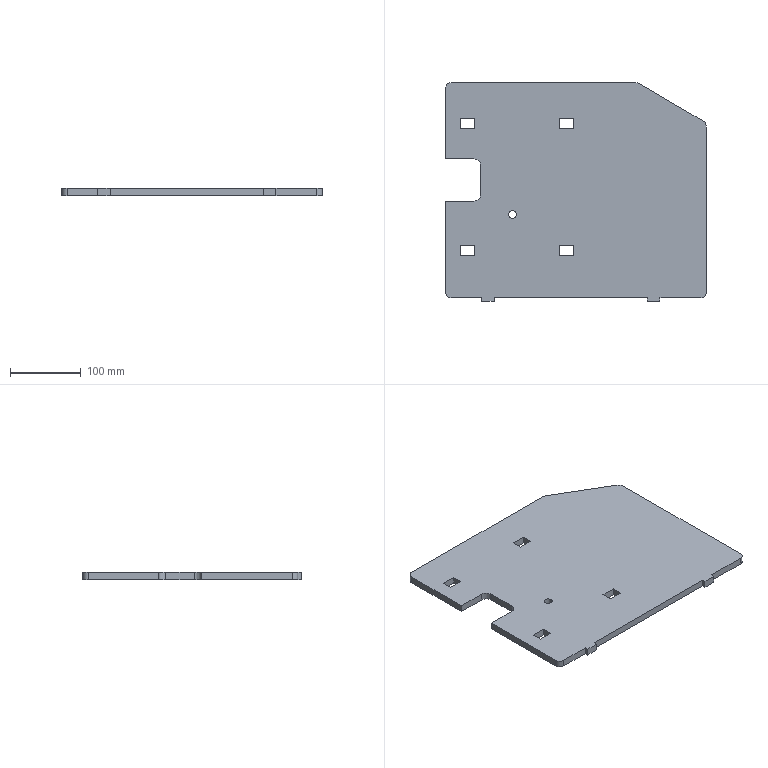Part | SolidWorks | features Extrusion 1 | 1 solid | 44 faces | box 370 x 310 x 10 mm | volume 1059963 mm3 | plane 35 | cylinder 9 | commonest cylinder face diameters 20 x4 16 x3 11 x2
STEP:
#1=CARTESIAN_POINT('',(352.502,683.941,10.));
#2=VERTEX_POINT('',#1);
#3=CARTESIAN_POINT('',(363.502,683.941,10.));
#4=VERTEX_POINT('',#3);
#5=CARTESIAN_POINT('',(358.002,683.941,10.));
#6=DIRECTION('',(0.,0.,1.));
#7=DIRECTION('',(1.,0.,0.));
#8=AXIS2_PLACEMENT_3D('',#5,#6,#7);
#9=CIRCLE('',#8,5.5);
#10=EDGE_CURVE('',#2,#4,#9,.T.);
#11=ORIENTED_EDGE('',*,*,#10,.T.);
#12=CARTESIAN_POINT('',(363.502,683.941,0.));
#13=VERTEX_POINT('',#12);
#14=CARTESIAN_POINT('',(363.502,683.941,10.));
#15=DIRECTION('',(0.,0.,-1.));
#16=VECTOR('',#15,1000.);
#17=LINE('',#14,#16);
#18=EDGE_CURVE('',#4,#13,#17,.T.);
#19=ORIENTED_EDGE('',*,*,#18,.T.);
#20=CARTESIAN_POINT('',(352.502,683.941,0.));
#21=VERTEX_POINT('',#20);
#22=CARTESIAN_POINT('',(358.002,683.941,0.));
#23=DIRECTION('',(0.,0.,1.));
#24=DIRECTION('',(1.,0.,0.));
#25=AXIS2_PLACEMENT_3D('',#22,#23,#24);
#26=CIRCLE('',#25,5.5);
#27=EDGE_CURVE('',#21,#13,#26,.T.);
#28=ORIENTED_EDGE('',*,*,#27,.F.);
#29=CARTESIAN_POINT('',(352.502,683.941,10.));
#30=DIRECTION('',(0.,0.,-1.));
#31=VECTOR('',#30,1000.);
#32=LINE('',#29,#31);
#33=EDGE_CURVE('',#2,#21,#32,.T.);
#34=ORIENTED_EDGE('',*,*,#33,.F.);
#35=EDGE_LOOP('',(#11,#19,#28,#34));
#36=FACE_OUTER_BOUND('',#35,.T.);
#37=CARTESIAN_POINT('',(358.002,683.941,10.));
#38=DIRECTION('',(0.,0.,-1.));
#39=DIRECTION('',(-1.,0.,0.));
#40=AXIS2_PLACEMENT_3D('',#37,#38,#39);
#41=CYLINDRICAL_SURFACE('',#40,5.5);
#42=ADVANCED_FACE('',(#36),#41,.F.);
#43=CARTESIAN_POINT('',(444.202,805.941,10.));
#44=VERTEX_POINT('',#43);
#45=CARTESIAN_POINT('',(444.202,820.141,10.));
#46=VERTEX_POINT('',#45);
#47=CARTESIAN_POINT('',(444.202,820.141,10.));
#48=DIRECTION('',(0.,1.,0.));
#49=VECTOR('',#48,1000.);
#50=LINE('',#47,#49);
#51=EDGE_CURVE('',#44,#46,#50,.T.);
#52=ORIENTED_EDGE('',*,*,#51,.F.);
#53=CARTESIAN_POINT('',(424.002,805.941,10.));
#54=VERTEX_POINT('',#53);
#55=CARTESIAN_POINT('',(444.202,805.941,10.));
#56=DIRECTION('',(1.,0.,0.));
#57=VECTOR('',#56,1000.);
#58=LINE('',#55,#57);
#59=EDGE_CURVE('',#54,#44,#58,.T.);
#60=ORIENTED_EDGE('',*,*,#59,.F.);
#61=CARTESIAN_POINT('',(424.002,820.141,10.));
#62=VERTEX_POINT('',#61);
#63=CARTESIAN_POINT('',(424.002,805.941,10.));
#64=DIRECTION('',(0.,-1.,0.));
#65=VECTOR('',#64,1000.);
#66=LINE('',#63,#65);
#67=EDGE_CURVE('',#62,#54,#66,.T.);
#68=ORIENTED_EDGE('',*,*,#67,.F.);
#69=CARTESIAN_POINT('',(424.002,820.141,10.));
#70=DIRECTION('',(-1.,0.,0.));
#71=VECTOR('',#70,1000.);
#72=LINE('',#69,#71);
#73=EDGE_CURVE('',#46,#62,#72,.T.);
#74=ORIENTED_EDGE('',*,*,#73,.F.);
#75=EDGE_LOOP('',(#52,#60,#68,#74));
#76=FACE_BOUND('',#75,.T.);
#77=CARTESIAN_POINT('',(304.202,805.941,10.));
#78=VERTEX_POINT('',#77);
#79=CARTESIAN_POINT('',(304.202,820.141,10.));
#80=VERTEX_POINT('',#79);
#81=CARTESIAN_POINT('',(304.202,820.141,10.));
#82=DIRECTION('',(0.,1.,0.));
#83=VECTOR('',#82,1000.);
#84=LINE('',#81,#83);
#85=EDGE_CURVE('',#78,#80,#84,.T.);
#86=ORIENTED_EDGE('',*,*,#85,.F.);
#87=CARTESIAN_POINT('',(284.002,805.941,10.));
#88=VERTEX_POINT('',#87);
#89=CARTESIAN_POINT('',(304.202,805.941,10.));
#90=DIRECTION('',(1.,0.,0.));
#91=VECTOR('',#90,1000.);
#92=LINE('',#89,#91);
#93=EDGE_CURVE('',#88,#78,#92,.T.);
#94=ORIENTED_EDGE('',*,*,#93,.F.);
#95=CARTESIAN_POINT('',(284.002,820.141,10.));
#96=VERTEX_POINT('',#95);
#97=CARTESIAN_POINT('',(284.002,805.941,10.));
#98=DIRECTION('',(0.,-1.,0.));
#99=VECTOR('',#98,1000.);
#100=LINE('',#97,#99);
#101=EDGE_CURVE('',#96,#88,#100,.T.);
#102=ORIENTED_EDGE('',*,*,#101,.F.);
#103=CARTESIAN_POINT('',(284.002,820.141,10.));
#104=DIRECTION('',(-1.,0.,0.));
#105=VECTOR('',#104,1000.);
#106=LINE('',#103,#105);
#107=EDGE_CURVE('',#80,#96,#106,.T.);
#108=ORIENTED_EDGE('',*,*,#107,.F.);
#109=EDGE_LOOP('',(#86,#94,#102,#108));
#110=FACE_BOUND('',#109,.T.);
#111=CARTESIAN_POINT('',(444.202,626.141,10.));
#112=VERTEX_POINT('',#111);
#113=CARTESIAN_POINT('',(444.202,640.341,10.));
#114=VERTEX_POINT('',#113);
#115=CARTESIAN_POINT('',(444.202,640.341,10.));
#116=DIRECTION('',(0.,1.,0.));
#117=VECTOR('',#116,1000.);
#118=LINE('',#115,#117);
#119=EDGE_CURVE('',#112,#114,#118,.T.);
#120=ORIENTED_EDGE('',*,*,#119,.F.);
#121=CARTESIAN_POINT('',(424.002,626.141,10.));
#122=VERTEX_POINT('',#121);
#123=CARTESIAN_POINT('',(444.202,626.141,10.));
#124=DIRECTION('',(1.,0.,0.));
#125=VECTOR('',#124,1000.);
#126=LINE('',#123,#125);
#127=EDGE_CURVE('',#122,#112,#126,.T.);
#128=ORIENTED_EDGE('',*,*,#127,.F.);
#129=CARTESIAN_POINT('',(424.002,640.341,10.));
#130=VERTEX_POINT('',#129);
#131=CARTESIAN_POINT('',(424.002,626.141,10.));
#132=DIRECTION('',(0.,-1.,0.));
#133=VECTOR('',#132,1000.);
#134=LINE('',#131,#133);
#135=EDGE_CURVE('',#130,#122,#134,.T.);
#136=ORIENTED_EDGE('',*,*,#135,.F.);
#137=CARTESIAN_POINT('',(424.002,640.341,10.));
#138=DIRECTION('',(-1.,0.,0.));
#139=VECTOR('',#138,1000.);
#140=LINE('',#137,#139);
#141=EDGE_CURVE('',#114,#130,#140,.T.);
#142=ORIENTED_EDGE('',*,*,#141,.F.);
#143=EDGE_LOOP('',(#120,#128,#136,#142));
#144=FACE_BOUND('',#143,.T.);
#145=CARTESIAN_POINT('',(304.202,626.141,10.));
#146=VERTEX_POINT('',#145);
#147=CARTESIAN_POINT('',(304.202,640.341,10.));
#148=VERTEX_POINT('',#147);
#149=CARTESIAN_POINT('',(304.202,640.341,10.));
#150=DIRECTION('',(0.,1.,0.));
#151=VECTOR('',#150,1000.);
#152=LINE('',#149,#151);
#153=EDGE_CURVE('',#146,#148,#152,.T.);
#154=ORIENTED_EDGE('',*,*,#153,.F.);
#155=CARTESIAN_POINT('',(284.002,626.141,10.));
#156=VERTEX_POINT('',#155);
#157=CARTESIAN_POINT('',(304.202,626.141,10.));
#158=DIRECTION('',(1.,0.,0.));
#159=VECTOR('',#158,1000.);
#160=LINE('',#157,#159);
#161=EDGE_CURVE('',#156,#146,#160,.T.);
#162=ORIENTED_EDGE('',*,*,#161,.F.);
#163=CARTESIAN_POINT('',(284.002,640.341,10.));
#164=VERTEX_POINT('',#163);
#165=CARTESIAN_POINT('',(284.002,626.141,10.));
#166=DIRECTION('',(0.,-1.,0.));
#167=VECTOR('',#166,1000.);
#168=LINE('',#165,#167);
#169=EDGE_CURVE('',#164,#156,#168,.T.);
#170=ORIENTED_EDGE('',*,*,#169,.F.);
#171=CARTESIAN_POINT('',(284.002,640.341,10.));
#172=DIRECTION('',(-1.,0.,0.));
#173=VECTOR('',#172,1000.);
#174=LINE('',#171,#173);
#175=EDGE_CURVE('',#148,#164,#174,.T.);
#176=ORIENTED_EDGE('',*,*,#175,.F.);
#177=EDGE_LOOP('',(#154,#162,#170,#176));
#178=FACE_BOUND('',#177,.T.);
#179=CARTESIAN_POINT('',(633.002,807.92,10.));
#180=VERTEX_POINT('',#179);
#181=CARTESIAN_POINT('',(628.108,816.518,10.));
#182=VERTEX_POINT('',#181);
#183=CARTESIAN_POINT('',(623.002,807.92,10.));
#184=DIRECTION('',(0.,0.,1.));
#185=DIRECTION('',(1.,0.,0.));
#186=AXIS2_PLACEMENT_3D('',#183,#184,#185);
#187=CIRCLE('',#186,10.);
#188=EDGE_CURVE('',#180,#182,#187,.T.);
#189=ORIENTED_EDGE('',*,*,#188,.T.);
#190=CARTESIAN_POINT('',(538.108,869.539,10.));
#191=VERTEX_POINT('',#190);
#192=CARTESIAN_POINT('',(538.108,869.539,10.));
#193=DIRECTION('',(-0.8616,0.5076,0.));
#194=VECTOR('',#193,1000.);
#195=LINE('',#192,#194);
#196=EDGE_CURVE('',#182,#191,#195,.T.);
#197=ORIENTED_EDGE('',*,*,#196,.T.);
#198=CARTESIAN_POINT('',(533.002,870.941,10.));
#199=VERTEX_POINT('',#198);
#200=CARTESIAN_POINT('',(533.002,860.941,10.));
#201=DIRECTION('',(0.,0.,1.));
#202=DIRECTION('',(1.,0.,0.));
#203=AXIS2_PLACEMENT_3D('',#200,#201,#202);
#204=CIRCLE('',#203,10.);
#205=EDGE_CURVE('',#191,#199,#204,.T.);
#206=ORIENTED_EDGE('',*,*,#205,.T.);
#207=CARTESIAN_POINT('',(271.002,870.941,10.));
#208=VERTEX_POINT('',#207);
#209=CARTESIAN_POINT('',(533.002,870.941,10.));
#210=DIRECTION('',(-1.,0.,0.));
#211=VECTOR('',#210,1000.);
#212=LINE('',#209,#211);
#213=EDGE_CURVE('',#199,#208,#212,.T.);
#214=ORIENTED_EDGE('',*,*,#213,.T.);
#215=CARTESIAN_POINT('',(263.002,862.941,10.));
#216=VERTEX_POINT('',#215);
#217=CARTESIAN_POINT('',(271.002,862.941,10.));
#218=DIRECTION('',(0.,0.,1.));
#219=DIRECTION('',(1.,0.,0.));
#220=AXIS2_PLACEMENT_3D('',#217,#218,#219);
#221=CIRCLE('',#220,8.);
#222=EDGE_CURVE('',#208,#216,#221,.T.);
#223=ORIENTED_EDGE('',*,*,#222,.T.);
#224=CARTESIAN_POINT('',(263.002,762.941,10.));
#225=VERTEX_POINT('',#224);
#226=CARTESIAN_POINT('',(263.002,862.941,10.));
#227=DIRECTION('',(0.,-1.,0.));
#228=VECTOR('',#227,1000.);
#229=LINE('',#226,#228);
#230=EDGE_CURVE('',#216,#225,#229,.T.);
#231=ORIENTED_EDGE('',*,*,#230,.T.);
#232=CARTESIAN_POINT('',(303.002,762.941,10.));
#233=VERTEX_POINT('',#232);
#234=CARTESIAN_POINT('',(263.002,762.941,10.));
#235=DIRECTION('',(1.,0.,0.));
#236=VECTOR('',#235,1000.);
#237=LINE('',#234,#236);
#238=EDGE_CURVE('',#225,#233,#237,.T.);
#239=ORIENTED_EDGE('',*,*,#238,.T.);
#240=CARTESIAN_POINT('',(313.002,752.941,10.));
#241=VERTEX_POINT('',#240);
#242=CARTESIAN_POINT('',(303.002,752.941,10.));
#243=DIRECTION('',(0.,0.,-1.));
#244=DIRECTION('',(1.,0.,0.));
#245=AXIS2_PLACEMENT_3D('',#242,#243,#244);
#246=CIRCLE('',#245,10.);
#247=EDGE_CURVE('',#233,#241,#246,.T.);
#248=ORIENTED_EDGE('',*,*,#247,.T.);
#249=CARTESIAN_POINT('',(313.002,712.941,10.));
#250=VERTEX_POINT('',#249);
#251=CARTESIAN_POINT('',(313.002,752.941,10.));
#252=DIRECTION('',(0.,-1.,0.));
#253=VECTOR('',#252,1000.);
#254=LINE('',#251,#253);
#255=EDGE_CURVE('',#241,#250,#254,.T.);
#256=ORIENTED_EDGE('',*,*,#255,.T.);
#257=CARTESIAN_POINT('',(303.002,702.941,10.));
#258=VERTEX_POINT('',#257);
#259=CARTESIAN_POINT('',(303.002,712.941,10.));
#260=DIRECTION('',(0.,0.,-1.));
#261=DIRECTION('',(1.,0.,0.));
#262=AXIS2_PLACEMENT_3D('',#259,#260,#261);
#263=CIRCLE('',#262,10.);
#264=EDGE_CURVE('',#250,#258,#263,.T.);
#265=ORIENTED_EDGE('',*,*,#264,.T.);
#266=CARTESIAN_POINT('',(263.002,702.941,10.));
#267=VERTEX_POINT('',#266);
#268=CARTESIAN_POINT('',(303.002,702.941,10.));
#269=DIRECTION('',(-1.,0.,0.));
#270=VECTOR('',#269,1000.);
#271=LINE('',#268,#270);
#272=EDGE_CURVE('',#258,#267,#271,.T.);
#273=ORIENTED_EDGE('',*,*,#272,.T.);
#274=CARTESIAN_POINT('',(263.002,573.941,10.));
#275=VERTEX_POINT('',#274);
#276=CARTESIAN_POINT('',(263.002,702.941,10.));
#277=DIRECTION('',(0.,-1.,0.));
#278=VECTOR('',#277,1000.);
#279=LINE('',#276,#278);
#280=EDGE_CURVE('',#267,#275,#279,.T.);
#281=ORIENTED_EDGE('',*,*,#280,.T.);
#282=CARTESIAN_POINT('',(271.002,565.941,10.));
#283=VERTEX_POINT('',#282);
#284=CARTESIAN_POINT('',(271.002,573.941,10.));
#285=DIRECTION('',(0.,0.,1.));
#286=DIRECTION('',(1.,0.,0.));
#287=AXIS2_PLACEMENT_3D('',#284,#285,#286);
#288=CIRCLE('',#287,8.);
#289=EDGE_CURVE('',#275,#283,#288,.T.);
#290=ORIENTED_EDGE('',*,*,#289,.T.);
#291=CARTESIAN_POINT('',(314.061,565.941,10.));
#292=VERTEX_POINT('',#291);
#293=CARTESIAN_POINT('',(271.002,565.941,10.));
#294=DIRECTION('',(1.,0.,0.));
#295=VECTOR('',#294,1000.);
#296=LINE('',#293,#295);
#297=EDGE_CURVE('',#283,#292,#296,.T.);
#298=ORIENTED_EDGE('',*,*,#297,.T.);
#299=CARTESIAN_POINT('',(314.061,560.941,10.));
#300=VERTEX_POINT('',#299);
#301=CARTESIAN_POINT('',(314.061,565.941,10.));
#302=DIRECTION('',(0.,-1.,0.));
#303=VECTOR('',#302,1000.);
#304=LINE('',#301,#303);
#305=EDGE_CURVE('',#292,#300,#304,.T.);
#306=ORIENTED_EDGE('',*,*,#305,.T.);
#307=CARTESIAN_POINT('',(332.061,560.941,10.));
#308=VERTEX_POINT('',#307);
#309=CARTESIAN_POINT('',(314.061,560.941,10.));
#310=DIRECTION('',(1.,0.,0.));
#311=VECTOR('',#310,1000.);
#312=LINE('',#309,#311);
#313=EDGE_CURVE('',#300,#308,#312,.T.);
#314=ORIENTED_EDGE('',*,*,#313,.T.);
#315=CARTESIAN_POINT('',(332.061,565.941,10.));
#316=VERTEX_POINT('',#315);
#317=CARTESIAN_POINT('',(332.061,560.941,10.));
#318=DIRECTION('',(0.,1.,0.));
#319=VECTOR('',#318,1000.);
#320=LINE('',#317,#319);
#321=EDGE_CURVE('',#308,#316,#320,.T.);
#322=ORIENTED_EDGE('',*,*,#321,.T.);
#323=CARTESIAN_POINT('',(549.061,565.941,10.));
#324=VERTEX_POINT('',#323);
#325=CARTESIAN_POINT('',(332.061,565.941,10.));
#326=DIRECTION('',(1.,0.,0.));
#327=VECTOR('',#326,1000.);
#328=LINE('',#325,#327);
#329=EDGE_CURVE('',#316,#324,#328,.T.);
#330=ORIENTED_EDGE('',*,*,#329,.T.);
#331=CARTESIAN_POINT('',(549.061,560.941,10.));
#332=VERTEX_POINT('',#331);
#333=CARTESIAN_POINT('',(549.061,565.941,10.));
#334=DIRECTION('',(0.,-1.,0.));
#335=VECTOR('',#334,1000.);
#336=LINE('',#333,#335);
#337=EDGE_CURVE('',#324,#332,#336,.T.);
#338=ORIENTED_EDGE('',*,*,#337,.T.);
#339=CARTESIAN_POINT('',(567.061,560.941,10.));
#340=VERTEX_POINT('',#339);
#341=CARTESIAN_POINT('',(549.061,560.941,10.));
#342=DIRECTION('',(1.,0.,0.));
#343=VECTOR('',#342,1000.);
#344=LINE('',#341,#343);
#345=EDGE_CURVE('',#332,#340,#344,.T.);
#346=ORIENTED_EDGE('',*,*,#345,.T.);
#347=CARTESIAN_POINT('',(567.061,565.941,10.));
#348=VERTEX_POINT('',#347);
#349=CARTESIAN_POINT('',(567.061,560.941,10.));
#350=DIRECTION('',(0.,1.,0.));
#351=VECTOR('',#350,1000.);
#352=LINE('',#349,#351);
#353=EDGE_CURVE('',#340,#348,#352,.T.);
#354=ORIENTED_EDGE('',*,*,#353,.T.);
#355=CARTESIAN_POINT('',(625.002,565.941,10.));
#356=VERTEX_POINT('',#355);
#357=CARTESIAN_POINT('',(567.061,565.941,10.));
#358=DIRECTION('',(1.,0.,0.));
#359=VECTOR('',#358,1000.);
#360=LINE('',#357,#359);
#361=EDGE_CURVE('',#348,#356,#360,.T.);
#362=ORIENTED_EDGE('',*,*,#361,.T.);
#363=CARTESIAN_POINT('',(633.002,573.941,10.));
#364=VERTEX_POINT('',#363);
#365=CARTESIAN_POINT('',(625.002,573.941,10.));
#366=DIRECTION('',(0.,0.,1.));
#367=DIRECTION('',(1.,0.,0.));
#368=AXIS2_PLACEMENT_3D('',#365,#366,#367);
#369=CIRCLE('',#368,8.);
#370=EDGE_CURVE('',#356,#364,#369,.T.);
#371=ORIENTED_EDGE('',*,*,#370,.T.);
#372=CARTESIAN_POINT('',(633.002,807.92,10.));
#373=DIRECTION('',(0.,1.,0.));
#374=VECTOR('',#373,1000.);
#375=LINE('',#372,#374);
#376=EDGE_CURVE('',#364,#180,#375,.T.);
#377=ORIENTED_EDGE('',*,*,#376,.T.);
#378=EDGE_LOOP('',(#189,#197,#206,#214,#223,#231,#239,#248,#256,#265,#273,#281,#290,#298,#306,#314,#322,#330,#338,#346,#354,#362,#371,#377));
#379=FACE_OUTER_BOUND('',#378,.T.);
#380=ORIENTED_EDGE('',*,*,#10,.F.);
#381=CARTESIAN_POINT('',(358.002,683.941,10.));
#382=DIRECTION('',(0.,0.,1.));
#383=DIRECTION('',(1.,0.,0.));
#384=AXIS2_PLACEMENT_3D('',#381,#382,#383);
#385=CIRCLE('',#384,5.5);
#386=EDGE_CURVE('',#4,#2,#385,.T.);
#387=ORIENTED_EDGE('',*,*,#386,.F.);
#388=EDGE_LOOP('',(#380,#387));
#389=FACE_BOUND('',#388,.T.);
#390=CARTESIAN_POINT('',(623.002,807.92,10.));
#391=DIRECTION('',(0.,0.,1.));
#392=DIRECTION('',(1.,0.,0.));
#393=AXIS2_PLACEMENT_3D('',#390,#391,#392);
#394=PLANE('',#393);
#395=ADVANCED_FACE('',(#76,#110,#144,#178,#379,#389),#394,.T.);
#396=CARTESIAN_POINT('',(284.002,805.941,0.));
#397=VERTEX_POINT('',#396);
#398=CARTESIAN_POINT('',(304.202,805.941,0.));
#399=VERTEX_POINT('',#398);
#400=CARTESIAN_POINT('',(304.202,805.941,0.));
#401=DIRECTION('',(1.,0.,0.));
#402=VECTOR('',#401,1000.);
#403=LINE('',#400,#402);
#404=EDGE_CURVE('',#397,#399,#403,.T.);
#405=ORIENTED_EDGE('',*,*,#404,.T.);
#406=CARTESIAN_POINT('',(304.202,820.141,0.));
#407=VERTEX_POINT('',#406);
#408=CARTESIAN_POINT('',(304.202,820.141,0.));
#409=DIRECTION('',(0.,1.,0.));
#410=VECTOR('',#409,1000.);
#411=LINE('',#408,#410);
#412=EDGE_CURVE('',#399,#407,#411,.T.);
#413=ORIENTED_EDGE('',*,*,#412,.T.);
#414=CARTESIAN_POINT('',(284.002,820.141,0.));
#415=VERTEX_POINT('',#414);
#416=CARTESIAN_POINT('',(284.002,820.141,0.));
#417=DIRECTION('',(-1.,0.,0.));
#418=VECTOR('',#417,1000.);
#419=LINE('',#416,#418);
#420=EDGE_CURVE('',#407,#415,#419,.T.);
#421=ORIENTED_EDGE('',*,*,#420,.T.);
#422=CARTESIAN_POINT('',(284.002,805.941,0.));
#423=DIRECTION('',(0.,-1.,0.));
#424=VECTOR('',#423,1000.);
#425=LINE('',#422,#424);
#426=EDGE_CURVE('',#415,#397,#425,.T.);
#427=ORIENTED_EDGE('',*,*,#426,.T.);
#428=EDGE_LOOP('',(#405,#413,#421,#427));
#429=FACE_BOUND('',#428,.T.);
#430=CARTESIAN_POINT('',(284.002,626.141,0.));
#431=VERTEX_POINT('',#430);
#432=CARTESIAN_POINT('',(304.202,626.141,0.));
#433=VERTEX_POINT('',#432);
#434=CARTESIAN_POINT('',(304.202,626.141,0.));
#435=DIRECTION('',(1.,0.,0.));
#436=VECTOR('',#435,1000.);
#437=LINE('',#434,#436);
#438=EDGE_CURVE('',#431,#433,#437,.T.);
#439=ORIENTED_EDGE('',*,*,#438,.T.);
#440=CARTESIAN_POINT('',(304.202,640.341,0.));
#441=VERTEX_POINT('',#440);
#442=CARTESIAN_POINT('',(304.202,640.341,0.));
#443=DIRECTION('',(0.,1.,0.));
#444=VECTOR('',#443,1000.);
#445=LINE('',#442,#444);
#446=EDGE_CURVE('',#433,#441,#445,.T.);
#447=ORIENTED_EDGE('',*,*,#446,.T.);
#448=CARTESIAN_POINT('',(284.002,640.341,0.));
#449=VERTEX_POINT('',#448);
#450=CARTESIAN_POINT('',(284.002,640.341,0.));
#451=DIRECTION('',(-1.,0.,0.));
#452=VECTOR('',#451,1000.);
#453=LINE('',#450,#452);
#454=EDGE_CURVE('',#441,#449,#453,.T.);
#455=ORIENTED_EDGE('',*,*,#454,.T.);
#456=CARTESIAN_POINT('',(284.002,626.141,0.));
#457=DIRECTION('',(0.,-1.,0.));
#458=VECTOR('',#457,1000.);
#459=LINE('',#456,#458);
#460=EDGE_CURVE('',#449,#431,#459,.T.);
#461=ORIENTED_EDGE('',*,*,#460,.T.);
#462=EDGE_LOOP('',(#439,#447,#455,#461));
#463=FACE_BOUND('',#462,.T.);
#464=CARTESIAN_POINT('',(633.002,807.92,0.));
#465=VERTEX_POINT('',#464);
#466=CARTESIAN_POINT('',(628.108,816.518,0.));
#467=VERTEX_POINT('',#466);
#468=CARTESIAN_POINT('',(623.002,807.92,0.));
#469=DIRECTION('',(0.,0.,1.));
#470=DIRECTION('',(1.,0.,0.));
#471=AXIS2_PLACEMENT_3D('',#468,#469,#470);
#472=CIRCLE('',#471,10.);
#473=EDGE_CURVE('',#465,#467,#472,.T.);
#474=ORIENTED_EDGE('',*,*,#473,.F.);
#475=CARTESIAN_POINT('',(633.002,573.941,0.));
#476=VERTEX_POINT('',#475);
#477=CARTESIAN_POINT('',(633.002,807.92,0.));
#478=DIRECTION('',(0.,1.,0.));
#479=VECTOR('',#478,1000.);
#480=LINE('',#477,#479);
#481=EDGE_CURVE('',#476,#465,#480,.T.);
#482=ORIENTED_EDGE('',*,*,#481,.F.);
#483=CARTESIAN_POINT('',(625.002,565.941,0.));
#484=VERTEX_POINT('',#483);
#485=CARTESIAN_POINT('',(625.002,573.941,0.));
#486=DIRECTION('',(0.,0.,1.));
#487=DIRECTION('',(1.,0.,0.));
#488=AXIS2_PLACEMENT_3D('',#485,#486,#487);
#489=CIRCLE('',#488,8.);
#490=EDGE_CURVE('',#484,#476,#489,.T.);
#491=ORIENTED_EDGE('',*,*,#490,.F.);
#492=CARTESIAN_POINT('',(567.061,565.941,0.));
#493=VERTEX_POINT('',#492);
#494=CARTESIAN_POINT('',(567.061,565.941,0.));
#495=DIRECTION('',(1.,0.,0.));
#496=VECTOR('',#495,1000.);
#497=LINE('',#494,#496);
#498=EDGE_CURVE('',#493,#484,#497,.T.);
#499=ORIENTED_EDGE('',*,*,#498,.F.);
#500=CARTESIAN_POINT('',(567.061,560.941,0.));
#501=VERTEX_POINT('',#500);
#502=CARTESIAN_POINT('',(567.061,560.941,0.));
#503=DIRECTION('',(0.,1.,0.));
#504=VECTOR('',#503,1000.);
#505=LINE('',#502,#504);
#506=EDGE_CURVE('',#501,#493,#505,.T.);
#507=ORIENTED_EDGE('',*,*,#506,.F.);
#508=CARTESIAN_POINT('',(549.061,560.941,0.));
#509=VERTEX_POINT('',#508);
#510=CARTESIAN_POINT('',(549.061,560.941,0.));
#511=DIRECTION('',(1.,0.,0.));
#512=VECTOR('',#511,1000.);
#513=LINE('',#510,#512);
#514=EDGE_CURVE('',#509,#501,#513,.T.);
#515=ORIENTED_EDGE('',*,*,#514,.F.);
#516=CARTESIAN_POINT('',(549.061,565.941,0.));
#517=VERTEX_POINT('',#516);
#518=CARTESIAN_POINT('',(549.061,565.941,0.));
#519=DIRECTION('',(0.,-1.,0.));
#520=VECTOR('',#519,1000.);
#521=LINE('',#518,#520);
#522=EDGE_CURVE('',#517,#509,#521,.T.);
#523=ORIENTED_EDGE('',*,*,#522,.F.);
#524=CARTESIAN_POINT('',(332.061,565.941,0.));
#525=VERTEX_POINT('',#524);
#526=CARTESIAN_POINT('',(332.061,565.941,0.));
#527=DIRECTION('',(1.,0.,0.));
#528=VECTOR('',#527,1000.);
#529=LINE('',#526,#528);
#530=EDGE_CURVE('',#525,#517,#529,.T.);
#531=ORIENTED_EDGE('',*,*,#530,.F.);
#532=CARTESIAN_POINT('',(332.061,560.941,0.));
#533=VERTEX_POINT('',#532);
#534=CARTESIAN_POINT('',(332.061,560.941,0.));
#535=DIRECTION('',(0.,1.,0.));
#536=VECTOR('',#535,1000.);
#537=LINE('',#534,#536);
#538=EDGE_CURVE('',#533,#525,#537,.T.);
#539=ORIENTED_EDGE('',*,*,#538,.F.);
#540=CARTESIAN_POINT('',(314.061,560.941,0.));
#541=VERTEX_POINT('',#540);
#542=CARTESIAN_POINT('',(314.061,560.941,0.));
#543=DIRECTION('',(1.,0.,0.));
#544=VECTOR('',#543,1000.);
#545=LINE('',#542,#544);
#546=EDGE_CURVE('',#541,#533,#545,.T.);
#547=ORIENTED_EDGE('',*,*,#546,.F.);
#548=CARTESIAN_POINT('',(314.061,565.941,0.));
#549=VERTEX_POINT('',#548);
#550=CARTESIAN_POINT('',(314.061,565.941,0.));
#551=DIRECTION('',(0.,-1.,0.));
#552=VECTOR('',#551,1000.);
#553=LINE('',#550,#552);
#554=EDGE_CURVE('',#549,#541,#553,.T.);
#555=ORIENTED_EDGE('',*,*,#554,.F.);
#556=CARTESIAN_POINT('',(271.002,565.941,0.));
#557=VERTEX_POINT('',#556);
#558=CARTESIAN_POINT('',(271.002,565.941,0.));
#559=DIRECTION('',(1.,0.,0.));
#560=VECTOR('',#559,1000.);
#561=LINE('',#558,#560);
#562=EDGE_CURVE('',#557,#549,#561,.T.);
#563=ORIENTED_EDGE('',*,*,#562,.F.);
#564=CARTESIAN_POINT('',(263.002,573.941,0.));
#565=VERTEX_POINT('',#564);
#566=CARTESIAN_POINT('',(271.002,573.941,0.));
#567=DIRECTION('',(0.,0.,1.));
#568=DIRECTION('',(1.,0.,0.));
#569=AXIS2_PLACEMENT_3D('',#566,#567,#568);
#570=CIRCLE('',#569,8.);
#571=EDGE_CURVE('',#565,#557,#570,.T.);
#572=ORIENTED_EDGE('',*,*,#571,.F.);
#573=CARTESIAN_POINT('',(263.002,702.941,0.));
#574=VERTEX_POINT('',#573);
#575=CARTESIAN_POINT('',(263.002,702.941,0.));
#576=DIRECTION('',(0.,-1.,0.));
#577=VECTOR('',#576,1000.);
#578=LINE('',#575,#577);
#579=EDGE_CURVE('',#574,#565,#578,.T.);
#580=ORIENTED_EDGE('',*,*,#579,.F.);
#581=CARTESIAN_POINT('',(303.002,702.941,0.));
#582=VERTEX_POINT('',#581);
#583=CARTESIAN_POINT('',(303.002,702.941,0.));
#584=DIRECTION('',(-1.,0.,0.));
#585=VECTOR('',#584,1000.);
#586=LINE('',#583,#585);
#587=EDGE_CURVE('',#582,#574,#586,.T.);
#588=ORIENTED_EDGE('',*,*,#587,.F.);
#589=CARTESIAN_POINT('',(313.002,712.941,0.));
#590=VERTEX_POINT('',#589);
#591=CARTESIAN_POINT('',(303.002,712.941,0.));
#592=DIRECTION('',(0.,0.,-1.));
#593=DIRECTION('',(1.,0.,0.));
#594=AXIS2_PLACEMENT_3D('',#591,#592,#593);
#595=CIRCLE('',#594,10.);
#596=EDGE_CURVE('',#590,#582,#595,.T.);
#597=ORIENTED_EDGE('',*,*,#596,.F.);
#598=CARTESIAN_POINT('',(313.002,752.941,0.));
#599=VERTEX_POINT('',#598);
#600=CARTESIAN_POINT('',(313.002,752.941,0.));
#601=DIRECTION('',(0.,-1.,0.));
#602=VECTOR('',#601,1000.);
#603=LINE('',#600,#602);
#604=EDGE_CURVE('',#599,#590,#603,.T.);
#605=ORIENTED_EDGE('',*,*,#604,.F.);
#606=CARTESIAN_POINT('',(303.002,762.941,0.));
#607=VERTEX_POINT('',#606);
#608=CARTESIAN_POINT('',(303.002,752.941,0.));
#609=DIRECTION('',(0.,0.,-1.));
#610=DIRECTION('',(1.,0.,0.));
#611=AXIS2_PLACEMENT_3D('',#608,#609,#610);
#612=CIRCLE('',#611,10.);
#613=EDGE_CURVE('',#607,#599,#612,.T.);
#614=ORIENTED_EDGE('',*,*,#613,.F.);
#615=CARTESIAN_POINT('',(263.002,762.941,0.));
#616=VERTEX_POINT('',#615);
#617=CARTESIAN_POINT('',(263.002,762.941,0.));
#618=DIRECTION('',(1.,0.,0.));
#619=VECTOR('',#618,1000.);
#620=LINE('',#617,#619);
#621=EDGE_CURVE('',#616,#607,#620,.T.);
#622=ORIENTED_EDGE('',*,*,#621,.F.);
#623=CARTESIAN_POINT('',(263.002,862.941,0.));
#624=VERTEX_POINT('',#623);
#625=CARTESIAN_POINT('',(263.002,862.941,0.));
#626=DIRECTION('',(0.,-1.,0.));
#627=VECTOR('',#626,1000.);
#628=LINE('',#625,#627);
#629=EDGE_CURVE('',#624,#616,#628,.T.);
#630=ORIENTED_EDGE('',*,*,#629,.F.);
#631=CARTESIAN_POINT('',(271.002,870.941,0.));
#632=VERTEX_POINT('',#631);
#633=CARTESIAN_POINT('',(271.002,862.941,0.));
#634=DIRECTION('',(0.,0.,1.));
#635=DIRECTION('',(1.,0.,0.));
#636=AXIS2_PLACEMENT_3D('',#633,#634,#635);
#637=CIRCLE('',#636,8.);
#638=EDGE_CURVE('',#632,#624,#637,.T.);
#639=ORIENTED_EDGE('',*,*,#638,.F.);
#640=CARTESIAN_POINT('',(533.002,870.941,0.));
#641=VERTEX_POINT('',#640);
#642=CARTESIAN_POINT('',(533.002,870.941,0.));
#643=DIRECTION('',(-1.,0.,0.));
#644=VECTOR('',#643,1000.);
#645=LINE('',#642,#644);
#646=EDGE_CURVE('',#641,#632,#645,.T.);
#647=ORIENTED_EDGE('',*,*,#646,.F.);
#648=CARTESIAN_POINT('',(538.108,869.539,0.));
#649=VERTEX_POINT('',#648);
#650=CARTESIAN_POINT('',(533.002,860.941,0.));
#651=DIRECTION('',(0.,0.,1.));
#652=DIRECTION('',(1.,0.,0.));
#653=AXIS2_PLACEMENT_3D('',#650,#651,#652);
#654=CIRCLE('',#653,10.);
#655=EDGE_CURVE('',#649,#641,#654,.T.);
#656=ORIENTED_EDGE('',*,*,#655,.F.);
#657=CARTESIAN_POINT('',(538.108,869.539,0.));
#658=DIRECTION('',(-0.8616,0.5076,0.));
#659=VECTOR('',#658,1000.);
#660=LINE('',#657,#659);
#661=EDGE_CURVE('',#467,#649,#660,.T.);
#662=ORIENTED_EDGE('',*,*,#661,.F.);
#663=EDGE_LOOP('',(#474,#482,#491,#499,#507,#515,#523,#531,#539,#547,#555,#563,#572,#580,#588,#597,#605,#614,#622,#630,#639,#647,#656,#662));
#664=FACE_OUTER_BOUND('',#663,.T.);
#665=CARTESIAN_POINT('',(424.002,626.141,0.));
#666=VERTEX_POINT('',#665);
#667=CARTESIAN_POINT('',(444.202,626.141,0.));
#668=VERTEX_POINT('',#667);
#669=CARTESIAN_POINT('',(444.202,626.141,0.));
#670=DIRECTION('',(1.,0.,0.));
#671=VECTOR('',#670,1000.);
#672=LINE('',#669,#671);
#673=EDGE_CURVE('',#666,#668,#672,.T.);
#674=ORIENTED_EDGE('',*,*,#673,.T.);
#675=CARTESIAN_POINT('',(444.202,640.341,0.));
#676=VERTEX_POINT('',#675);
#677=CARTESIAN_POINT('',(444.202,640.341,0.));
#678=DIRECTION('',(0.,1.,0.));
#679=VECTOR('',#678,1000.);
#680=LINE('',#677,#679);
#681=EDGE_CURVE('',#668,#676,#680,.T.);
#682=ORIENTED_EDGE('',*,*,#681,.T.);
#683=CARTESIAN_POINT('',(424.002,640.341,0.));
#684=VERTEX_POINT('',#683);
#685=CARTESIAN_POINT('',(424.002,640.341,0.));
#686=DIRECTION('',(-1.,0.,0.));
#687=VECTOR('',#686,1000.);
#688=LINE('',#685,#687);
#689=EDGE_CURVE('',#676,#684,#688,.T.);
#690=ORIENTED_EDGE('',*,*,#689,.T.);
#691=CARTESIAN_POINT('',(424.002,626.141,0.));
#692=DIRECTION('',(0.,-1.,0.));
#693=VECTOR('',#692,1000.);
#694=LINE('',#691,#693);
#695=EDGE_CURVE('',#684,#666,#694,.T.);
#696=ORIENTED_EDGE('',*,*,#695,.T.);
#697=EDGE_LOOP('',(#674,#682,#690,#696));
#698=FACE_BOUND('',#697,.T.);
#699=CARTESIAN_POINT('',(424.002,805.941,0.));
#700=VERTEX_POINT('',#699);
#701=CARTESIAN_POINT('',(444.202,805.941,0.));
#702=VERTEX_POINT('',#701);
#703=CARTESIAN_POINT('',(444.202,805.941,0.));
#704=DIRECTION('',(1.,0.,0.));
#705=VECTOR('',#704,1000.);
#706=LINE('',#703,#705);
#707=EDGE_CURVE('',#700,#702,#706,.T.);
#708=ORIENTED_EDGE('',*,*,#707,.T.);
#709=CARTESIAN_POINT('',(444.202,820.141,0.));
#710=VERTEX_POINT('',#709);
#711=CARTESIAN_POINT('',(444.202,820.141,0.));
#712=DIRECTION('',(0.,1.,0.));
#713=VECTOR('',#712,1000.);
#714=LINE('',#711,#713);
#715=EDGE_CURVE('',#702,#710,#714,.T.);
#716=ORIENTED_EDGE('',*,*,#715,.T.);
#717=CARTESIAN_POINT('',(424.002,820.141,0.));
#718=VERTEX_POINT('',#717);
#719=CARTESIAN_POINT('',(424.002,820.141,0.));
#720=DIRECTION('',(-1.,0.,0.));
#721=VECTOR('',#720,1000.);
#722=LINE('',#719,#721);
#723=EDGE_CURVE('',#710,#718,#722,.T.);
#724=ORIENTED_EDGE('',*,*,#723,.T.);
#725=CARTESIAN_POINT('',(424.002,805.941,0.));
#726=DIRECTION('',(0.,-1.,0.));
#727=VECTOR('',#726,1000.);
#728=LINE('',#725,#727);
#729=EDGE_CURVE('',#718,#700,#728,.T.);
#730=ORIENTED_EDGE('',*,*,#729,.T.);
#731=EDGE_LOOP('',(#708,#716,#724,#730));
#732=FACE_BOUND('',#731,.T.);
#733=ORIENTED_EDGE('',*,*,#27,.T.);
#734=CARTESIAN_POINT('',(358.002,683.941,0.));
#735=DIRECTION('',(0.,0.,1.));
#736=DIRECTION('',(1.,0.,0.));
#737=AXIS2_PLACEMENT_3D('',#734,#735,#736);
#738=CIRCLE('',#737,5.5);
#739=EDGE_CURVE('',#13,#21,#738,.T.);
#740=ORIENTED_EDGE('',*,*,#739,.T.);
#741=EDGE_LOOP('',(#733,#740));
#742=FACE_BOUND('',#741,.T.);
#743=CARTESIAN_POINT('',(623.002,807.92,0.));
#744=DIRECTION('',(0.,0.,1.));
#745=DIRECTION('',(1.,0.,0.));
#746=AXIS2_PLACEMENT_3D('',#743,#744,#745);
#747=PLANE('',#746);
#748=ADVANCED_FACE('',(#429,#463,#664,#698,#732,#742),#747,.F.);
#749=ORIENTED_EDGE('',*,*,#473,.T.);
#750=CARTESIAN_POINT('',(628.108,816.518,10.));
#751=DIRECTION('',(0.,0.,-1.));
#752=VECTOR('',#751,1000.);
#753=LINE('',#750,#752);
#754=EDGE_CURVE('',#182,#467,#753,.T.);
#755=ORIENTED_EDGE('',*,*,#754,.F.);
#756=ORIENTED_EDGE('',*,*,#188,.F.);
#757=CARTESIAN_POINT('',(633.002,807.92,10.));
#758=DIRECTION('',(0.,0.,-1.));
#759=VECTOR('',#758,1000.);
#760=LINE('',#757,#759);
#761=EDGE_CURVE('',#180,#465,#760,.T.);
#762=ORIENTED_EDGE('',*,*,#761,.T.);
#763=EDGE_LOOP('',(#749,#755,#756,#762));
#764=FACE_OUTER_BOUND('',#763,.T.);
#765=CARTESIAN_POINT('',(623.002,807.92,10.));
#766=DIRECTION('',(0.,0.,-1.));
#767=DIRECTION('',(-1.,0.,0.));
#768=AXIS2_PLACEMENT_3D('',#765,#766,#767);
#769=CYLINDRICAL_SURFACE('',#768,10.);
#770=ADVANCED_FACE('',(#764),#769,.T.);
#771=ORIENTED_EDGE('',*,*,#661,.T.);
#772=CARTESIAN_POINT('',(538.108,869.539,10.));
#773=DIRECTION('',(0.,0.,-1.));
#774=VECTOR('',#773,1000.);
#775=LINE('',#772,#774);
#776=EDGE_CURVE('',#191,#649,#775,.T.);
#777=ORIENTED_EDGE('',*,*,#776,.F.);
#778=ORIENTED_EDGE('',*,*,#196,.F.);
#779=ORIENTED_EDGE('',*,*,#754,.T.);
#780=EDGE_LOOP('',(#771,#777,#778,#779));
#781=FACE_OUTER_BOUND('',#780,.T.);
#782=CARTESIAN_POINT('',(538.108,869.539,10.));
#783=DIRECTION('',(-0.5076,-0.8616,0.));
#784=DIRECTION('',(0.8616,-0.5076,0.));
#785=AXIS2_PLACEMENT_3D('',#782,#783,#784);
#786=PLANE('',#785);
#787=ADVANCED_FACE('',(#781),#786,.F.);
#788=ORIENTED_EDGE('',*,*,#655,.T.);
#789=CARTESIAN_POINT('',(533.002,870.941,10.));
#790=DIRECTION('',(0.,0.,-1.));
#791=VECTOR('',#790,1000.);
#792=LINE('',#789,#791);
#793=EDGE_CURVE('',#199,#641,#792,.T.);
#794=ORIENTED_EDGE('',*,*,#793,.F.);
#795=ORIENTED_EDGE('',*,*,#205,.F.);
#796=ORIENTED_EDGE('',*,*,#776,.T.);
#797=EDGE_LOOP('',(#788,#794,#795,#796));
#798=FACE_OUTER_BOUND('',#797,.T.);
#799=CARTESIAN_POINT('',(533.002,860.941,10.));
#800=DIRECTION('',(0.,0.,-1.));
#801=DIRECTION('',(-1.,0.,0.));
#802=AXIS2_PLACEMENT_3D('',#799,#800,#801);
#803=CYLINDRICAL_SURFACE('',#802,10.);
#804=ADVANCED_FACE('',(#798),#803,.T.);
#805=ORIENTED_EDGE('',*,*,#646,.T.);
#806=CARTESIAN_POINT('',(271.002,870.941,10.));
#807=DIRECTION('',(0.,0.,-1.));
#808=VECTOR('',#807,1000.);
#809=LINE('',#806,#808);
#810=EDGE_CURVE('',#208,#632,#809,.T.);
#811=ORIENTED_EDGE('',*,*,#810,.F.);
#812=ORIENTED_EDGE('',*,*,#213,.F.);
#813=ORIENTED_EDGE('',*,*,#793,.T.);
#814=EDGE_LOOP('',(#805,#811,#812,#813));
#815=FACE_OUTER_BOUND('',#814,.T.);
#816=CARTESIAN_POINT('',(533.002,870.941,10.));
#817=DIRECTION('',(0.,-1.,0.));
#818=DIRECTION('',(1.,0.,0.));
#819=AXIS2_PLACEMENT_3D('',#816,#817,#818);
#820=PLANE('',#819);
#821=ADVANCED_FACE('',(#815),#820,.F.);
#822=ORIENTED_EDGE('',*,*,#638,.T.);
#823=CARTESIAN_POINT('',(263.002,862.941,10.));
#824=DIRECTION('',(0.,0.,-1.));
#825=VECTOR('',#824,1000.);
#826=LINE('',#823,#825);
#827=EDGE_CURVE('',#216,#624,#826,.T.);
#828=ORIENTED_EDGE('',*,*,#827,.F.);
#829=ORIENTED_EDGE('',*,*,#222,.F.);
#830=ORIENTED_EDGE('',*,*,#810,.T.);
#831=EDGE_LOOP('',(#822,#828,#829,#830));
#832=FACE_OUTER_BOUND('',#831,.T.);
#833=CARTESIAN_POINT('',(271.002,862.941,10.));
#834=DIRECTION('',(0.,0.,-1.));
#835=DIRECTION('',(-1.,0.,0.));
#836=AXIS2_PLACEMENT_3D('',#833,#834,#835);
#837=CYLINDRICAL_SURFACE('',#836,8.);
#838=ADVANCED_FACE('',(#832),#837,.T.);
#839=ORIENTED_EDGE('',*,*,#629,.T.);
#840=CARTESIAN_POINT('',(263.002,762.941,10.));
#841=DIRECTION('',(0.,0.,-1.));
#842=VECTOR('',#841,1000.);
#843=LINE('',#840,#842);
#844=EDGE_CURVE('',#225,#616,#843,.T.);
#845=ORIENTED_EDGE('',*,*,#844,.F.);
#846=ORIENTED_EDGE('',*,*,#230,.F.);
#847=ORIENTED_EDGE('',*,*,#827,.T.);
#848=EDGE_LOOP('',(#839,#845,#846,#847));
#849=FACE_OUTER_BOUND('',#848,.T.);
#850=CARTESIAN_POINT('',(263.002,862.941,10.));
#851=DIRECTION('',(1.,0.,0.));
#852=DIRECTION('',(0.,1.,0.));
#853=AXIS2_PLACEMENT_3D('',#850,#851,#852);
#854=PLANE('',#853);
#855=ADVANCED_FACE('',(#849),#854,.F.);
#856=ORIENTED_EDGE('',*,*,#621,.T.);
#857=CARTESIAN_POINT('',(303.002,762.941,10.));
#858=DIRECTION('',(0.,0.,-1.));
#859=VECTOR('',#858,1000.);
#860=LINE('',#857,#859);
#861=EDGE_CURVE('',#233,#607,#860,.T.);
#862=ORIENTED_EDGE('',*,*,#861,.F.);
#863=ORIENTED_EDGE('',*,*,#238,.F.);
#864=ORIENTED_EDGE('',*,*,#844,.T.);
#865=EDGE_LOOP('',(#856,#862,#863,#864));
#866=FACE_OUTER_BOUND('',#865,.T.);
#867=CARTESIAN_POINT('',(263.002,762.941,10.));
#868=DIRECTION('',(0.,1.,0.));
#869=DIRECTION('',(0.,0.,1.));
#870=AXIS2_PLACEMENT_3D('',#867,#868,#869);
#871=PLANE('',#870);
#872=ADVANCED_FACE('',(#866),#871,.F.);
#873=ORIENTED_EDGE('',*,*,#613,.T.);
#874=CARTESIAN_POINT('',(313.002,752.941,10.));
#875=DIRECTION('',(0.,0.,-1.));
#876=VECTOR('',#875,1000.);
#877=LINE('',#874,#876);
#878=EDGE_CURVE('',#241,#599,#877,.T.);
#879=ORIENTED_EDGE('',*,*,#878,.F.);
#880=ORIENTED_EDGE('',*,*,#247,.F.);
#881=ORIENTED_EDGE('',*,*,#861,.T.);
#882=EDGE_LOOP('',(#873,#879,#880,#881));
#883=FACE_OUTER_BOUND('',#882,.T.);
#884=CARTESIAN_POINT('',(303.002,752.941,10.));
#885=DIRECTION('',(0.,0.,-1.));
#886=DIRECTION('',(-1.,0.,0.));
#887=AXIS2_PLACEMENT_3D('',#884,#885,#886);
#888=CYLINDRICAL_SURFACE('',#887,10.);
#889=ADVANCED_FACE('',(#883),#888,.F.);
#890=ORIENTED_EDGE('',*,*,#604,.T.);
#891=CARTESIAN_POINT('',(313.002,712.941,10.));
#892=DIRECTION('',(0.,0.,-1.));
#893=VECTOR('',#892,1000.);
#894=LINE('',#891,#893);
#895=EDGE_CURVE('',#250,#590,#894,.T.);
#896=ORIENTED_EDGE('',*,*,#895,.F.);
#897=ORIENTED_EDGE('',*,*,#255,.F.);
#898=ORIENTED_EDGE('',*,*,#878,.T.);
#899=EDGE_LOOP('',(#890,#896,#897,#898));
#900=FACE_OUTER_BOUND('',#899,.T.);
#901=CARTESIAN_POINT('',(313.002,752.941,10.));
#902=DIRECTION('',(1.,0.,0.));
#903=DIRECTION('',(0.,0.,-1.));
#904=AXIS2_PLACEMENT_3D('',#901,#902,#903);
#905=PLANE('',#904);
#906=ADVANCED_FACE('',(#900),#905,.F.);
#907=ORIENTED_EDGE('',*,*,#596,.T.);
#908=CARTESIAN_POINT('',(303.002,702.941,10.));
#909=DIRECTION('',(0.,0.,-1.));
#910=VECTOR('',#909,1000.);
#911=LINE('',#908,#910);
#912=EDGE_CURVE('',#258,#582,#911,.T.);
#913=ORIENTED_EDGE('',*,*,#912,.F.);
#914=ORIENTED_EDGE('',*,*,#264,.F.);
#915=ORIENTED_EDGE('',*,*,#895,.T.);
#916=EDGE_LOOP('',(#907,#913,#914,#915));
#917=FACE_OUTER_BOUND('',#916,.T.);
#918=CARTESIAN_POINT('',(303.002,712.941,10.));
#919=DIRECTION('',(0.,0.,-1.));
#920=DIRECTION('',(-1.,0.,0.));
#921=AXIS2_PLACEMENT_3D('',#918,#919,#920);
#922=CYLINDRICAL_SURFACE('',#921,10.);
#923=ADVANCED_FACE('',(#917),#922,.F.);
#924=ORIENTED_EDGE('',*,*,#587,.T.);
#925=CARTESIAN_POINT('',(263.002,702.941,10.));
#926=DIRECTION('',(0.,0.,-1.));
#927=VECTOR('',#926,1000.);
#928=LINE('',#925,#927);
#929=EDGE_CURVE('',#267,#574,#928,.T.);
#930=ORIENTED_EDGE('',*,*,#929,.F.);
#931=ORIENTED_EDGE('',*,*,#272,.F.);
#932=ORIENTED_EDGE('',*,*,#912,.T.);
#933=EDGE_LOOP('',(#924,#930,#931,#932));
#934=FACE_OUTER_BOUND('',#933,.T.);
#935=CARTESIAN_POINT('',(303.002,702.941,10.));
#936=DIRECTION('',(0.,-1.,0.));
#937=DIRECTION('',(0.,0.,-1.));
#938=AXIS2_PLACEMENT_3D('',#935,#936,#937);
#939=PLANE('',#938);
#940=ADVANCED_FACE('',(#934),#939,.F.);
#941=ORIENTED_EDGE('',*,*,#579,.T.);
#942=CARTESIAN_POINT('',(263.002,573.941,10.));
#943=DIRECTION('',(0.,0.,-1.));
#944=VECTOR('',#943,1000.);
#945=LINE('',#942,#944);
#946=EDGE_CURVE('',#275,#565,#945,.T.);
#947=ORIENTED_EDGE('',*,*,#946,.F.);
#948=ORIENTED_EDGE('',*,*,#280,.F.);
#949=ORIENTED_EDGE('',*,*,#929,.T.);
#950=EDGE_LOOP('',(#941,#947,#948,#949));
#951=FACE_OUTER_BOUND('',#950,.T.);
#952=CARTESIAN_POINT('',(263.002,702.941,10.));
#953=DIRECTION('',(1.,0.,0.));
#954=DIRECTION('',(0.,1.,0.));
#955=AXIS2_PLACEMENT_3D('',#952,#953,#954);
#956=PLANE('',#955);
#957=ADVANCED_FACE('',(#951),#956,.F.);
#958=ORIENTED_EDGE('',*,*,#571,.T.);
#959=CARTESIAN_POINT('',(271.002,565.941,10.));
#960=DIRECTION('',(0.,0.,-1.));
#961=VECTOR('',#960,1000.);
#962=LINE('',#959,#961);
#963=EDGE_CURVE('',#283,#557,#962,.T.);
#964=ORIENTED_EDGE('',*,*,#963,.F.);
#965=ORIENTED_EDGE('',*,*,#289,.F.);
#966=ORIENTED_EDGE('',*,*,#946,.T.);
#967=EDGE_LOOP('',(#958,#964,#965,#966));
#968=FACE_OUTER_BOUND('',#967,.T.);
#969=CARTESIAN_POINT('',(271.002,573.941,10.));
#970=DIRECTION('',(0.,0.,-1.));
#971=DIRECTION('',(-1.,0.,0.));
#972=AXIS2_PLACEMENT_3D('',#969,#970,#971);
#973=CYLINDRICAL_SURFACE('',#972,8.);
#974=ADVANCED_FACE('',(#968),#973,.T.);
#975=ORIENTED_EDGE('',*,*,#562,.T.);
#976=CARTESIAN_POINT('',(314.061,565.941,10.));
#977=DIRECTION('',(0.,0.,-1.));
#978=VECTOR('',#977,1000.);
#979=LINE('',#976,#978);
#980=EDGE_CURVE('',#292,#549,#979,.T.);
#981=ORIENTED_EDGE('',*,*,#980,.F.);
#982=ORIENTED_EDGE('',*,*,#297,.F.);
#983=ORIENTED_EDGE('',*,*,#963,.T.);
#984=EDGE_LOOP('',(#975,#981,#982,#983));
#985=FACE_OUTER_BOUND('',#984,.T.);
#986=CARTESIAN_POINT('',(271.002,565.941,10.));
#987=DIRECTION('',(0.,1.,0.));
#988=DIRECTION('',(0.,0.,1.));
#989=AXIS2_PLACEMENT_3D('',#986,#987,#988);
#990=PLANE('',#989);
#991=ADVANCED_FACE('',(#985),#990,.F.);
#992=ORIENTED_EDGE('',*,*,#554,.T.);
#993=CARTESIAN_POINT('',(314.061,560.941,10.));
#994=DIRECTION('',(0.,0.,-1.));
#995=VECTOR('',#994,1000.);
#996=LINE('',#993,#995);
#997=EDGE_CURVE('',#300,#541,#996,.T.);
#998=ORIENTED_EDGE('',*,*,#997,.F.);
#999=ORIENTED_EDGE('',*,*,#305,.F.);
#1000=ORIENTED_EDGE('',*,*,#980,.T.);
#1001=EDGE_LOOP('',(#992,#998,#999,#1000));
#1002=FACE_OUTER_BOUND('',#1001,.T.);
#1003=CARTESIAN_POINT('',(314.061,565.941,10.));
#1004=DIRECTION('',(1.,0.,0.));
#1005=DIRECTION('',(0.,0.,-1.));
#1006=AXIS2_PLACEMENT_3D('',#1003,#1004,#1005);
#1007=PLANE('',#1006);
#1008=ADVANCED_FACE('',(#1002),#1007,.F.);
#1009=ORIENTED_EDGE('',*,*,#546,.T.);
#1010=CARTESIAN_POINT('',(332.061,560.941,10.));
#1011=DIRECTION('',(0.,0.,-1.));
#1012=VECTOR('',#1011,1000.);
#1013=LINE('',#1010,#1012);
#1014=EDGE_CURVE('',#308,#533,#1013,.T.);
#1015=ORIENTED_EDGE('',*,*,#1014,.F.);
#1016=ORIENTED_EDGE('',*,*,#313,.F.);
#1017=ORIENTED_EDGE('',*,*,#997,.T.);
#1018=EDGE_LOOP('',(#1009,#1015,#1016,#1017));
#1019=FACE_OUTER_BOUND('',#1018,.T.);
#1020=CARTESIAN_POINT('',(314.061,560.941,10.));
#1021=DIRECTION('',(0.,1.,0.));
#1022=DIRECTION('',(0.,0.,1.));
#1023=AXIS2_PLACEMENT_3D('',#1020,#1021,#1022);
#1024=PLANE('',#1023);
#1025=ADVANCED_FACE('',(#1019),#1024,.F.);
#1026=ORIENTED_EDGE('',*,*,#538,.T.);
#1027=CARTESIAN_POINT('',(332.061,565.941,10.));
#1028=DIRECTION('',(0.,0.,-1.));
#1029=VECTOR('',#1028,1000.);
#1030=LINE('',#1027,#1029);
#1031=EDGE_CURVE('',#316,#525,#1030,.T.);
#1032=ORIENTED_EDGE('',*,*,#1031,.F.);
#1033=ORIENTED_EDGE('',*,*,#321,.F.);
#1034=ORIENTED_EDGE('',*,*,#1014,.T.);
#1035=EDGE_LOOP('',(#1026,#1032,#1033,#1034));
#1036=FACE_OUTER_BOUND('',#1035,.T.);
#1037=CARTESIAN_POINT('',(332.061,560.941,10.));
#1038=DIRECTION('',(-1.,0.,0.));
#1039=DIRECTION('',(0.,0.,1.));
#1040=AXIS2_PLACEMENT_3D('',#1037,#1038,#1039);
#1041=PLANE('',#1040);
#1042=ADVANCED_FACE('',(#1036),#1041,.F.);
#1043=ORIENTED_EDGE('',*,*,#530,.T.);
#1044=CARTESIAN_POINT('',(549.061,565.941,10.));
#1045=DIRECTION('',(0.,0.,-1.));
#1046=VECTOR('',#1045,1000.);
#1047=LINE('',#1044,#1046);
#1048=EDGE_CURVE('',#324,#517,#1047,.T.);
#1049=ORIENTED_EDGE('',*,*,#1048,.F.);
#1050=ORIENTED_EDGE('',*,*,#329,.F.);
#1051=ORIENTED_EDGE('',*,*,#1031,.T.);
#1052=EDGE_LOOP('',(#1043,#1049,#1050,#1051));
#1053=FACE_OUTER_BOUND('',#1052,.T.);
#1054=CARTESIAN_POINT('',(332.061,565.941,10.));
#1055=DIRECTION('',(0.,1.,0.));
#1056=DIRECTION('',(0.,0.,1.));
#1057=AXIS2_PLACEMENT_3D('',#1054,#1055,#1056);
#1058=PLANE('',#1057);
#1059=ADVANCED_FACE('',(#1053),#1058,.F.);
#1060=ORIENTED_EDGE('',*,*,#522,.T.);
#1061=CARTESIAN_POINT('',(549.061,560.941,10.));
#1062=DIRECTION('',(0.,0.,-1.));
#1063=VECTOR('',#1062,1000.);
#1064=LINE('',#1061,#1063);
#1065=EDGE_CURVE('',#332,#509,#1064,.T.);
#1066=ORIENTED_EDGE('',*,*,#1065,.F.);
#1067=ORIENTED_EDGE('',*,*,#337,.F.);
#1068=ORIENTED_EDGE('',*,*,#1048,.T.);
#1069=EDGE_LOOP('',(#1060,#1066,#1067,#1068));
#1070=FACE_OUTER_BOUND('',#1069,.T.);
#1071=CARTESIAN_POINT('',(549.061,565.941,10.));
#1072=DIRECTION('',(1.,0.,0.));
#1073=DIRECTION('',(0.,0.,-1.));
#1074=AXIS2_PLACEMENT_3D('',#1071,#1072,#1073);
#1075=PLANE('',#1074);
#1076=ADVANCED_FACE('',(#1070),#1075,.F.);
#1077=ORIENTED_EDGE('',*,*,#514,.T.);
#1078=CARTESIAN_POINT('',(567.061,560.941,10.));
#1079=DIRECTION('',(0.,0.,-1.));
#1080=VECTOR('',#1079,1000.);
#1081=LINE('',#1078,#1080);
#1082=EDGE_CURVE('',#340,#501,#1081,.T.);
#1083=ORIENTED_EDGE('',*,*,#1082,.F.);
#1084=ORIENTED_EDGE('',*,*,#345,.F.);
#1085=ORIENTED_EDGE('',*,*,#1065,.T.);
#1086=EDGE_LOOP('',(#1077,#1083,#1084,#1085));
#1087=FACE_OUTER_BOUND('',#1086,.T.);
#1088=CARTESIAN_POINT('',(549.061,560.941,10.));
#1089=DIRECTION('',(0.,1.,0.));
#1090=DIRECTION('',(0.,0.,1.));
#1091=AXIS2_PLACEMENT_3D('',#1088,#1089,#1090);
#1092=PLANE('',#1091);
#1093=ADVANCED_FACE('',(#1087),#1092,.F.);
#1094=ORIENTED_EDGE('',*,*,#506,.T.);
#1095=CARTESIAN_POINT('',(567.061,565.941,10.));
#1096=DIRECTION('',(0.,0.,-1.));
#1097=VECTOR('',#1096,1000.);
#1098=LINE('',#1095,#1097);
#1099=EDGE_CURVE('',#348,#493,#1098,.T.);
#1100=ORIENTED_EDGE('',*,*,#1099,.F.);
#1101=ORIENTED_EDGE('',*,*,#353,.F.);
#1102=ORIENTED_EDGE('',*,*,#1082,.T.);
#1103=EDGE_LOOP('',(#1094,#1100,#1101,#1102));
#1104=FACE_OUTER_BOUND('',#1103,.T.);
#1105=CARTESIAN_POINT('',(567.061,560.941,10.));
#1106=DIRECTION('',(-1.,0.,0.));
#1107=DIRECTION('',(0.,0.,1.));
#1108=AXIS2_PLACEMENT_3D('',#1105,#1106,#1107);
#1109=PLANE('',#1108);
#1110=ADVANCED_FACE('',(#1104),#1109,.F.);
#1111=ORIENTED_EDGE('',*,*,#498,.T.);
#1112=CARTESIAN_POINT('',(625.002,565.941,10.));
#1113=DIRECTION('',(0.,0.,-1.));
#1114=VECTOR('',#1113,1000.);
#1115=LINE('',#1112,#1114);
#1116=EDGE_CURVE('',#356,#484,#1115,.T.);
#1117=ORIENTED_EDGE('',*,*,#1116,.F.);
#1118=ORIENTED_EDGE('',*,*,#361,.F.);
#1119=ORIENTED_EDGE('',*,*,#1099,.T.);
#1120=EDGE_LOOP('',(#1111,#1117,#1118,#1119));
#1121=FACE_OUTER_BOUND('',#1120,.T.);
#1122=CARTESIAN_POINT('',(567.061,565.941,10.));
#1123=DIRECTION('',(0.,1.,0.));
#1124=DIRECTION('',(0.,0.,1.));
#1125=AXIS2_PLACEMENT_3D('',#1122,#1123,#1124);
#1126=PLANE('',#1125);
#1127=ADVANCED_FACE('',(#1121),#1126,.F.);
#1128=ORIENTED_EDGE('',*,*,#490,.T.);
#1129=CARTESIAN_POINT('',(633.002,573.941,10.));
#1130=DIRECTION('',(0.,0.,-1.));
#1131=VECTOR('',#1130,1000.);
#1132=LINE('',#1129,#1131);
#1133=EDGE_CURVE('',#364,#476,#1132,.T.);
#1134=ORIENTED_EDGE('',*,*,#1133,.F.);
#1135=ORIENTED_EDGE('',*,*,#370,.F.);
#1136=ORIENTED_EDGE('',*,*,#1116,.T.);
#1137=EDGE_LOOP('',(#1128,#1134,#1135,#1136));
#1138=FACE_OUTER_BOUND('',#1137,.T.);
#1139=CARTESIAN_POINT('',(625.002,573.941,10.));
#1140=DIRECTION('',(0.,0.,-1.));
#1141=DIRECTION('',(-1.,0.,0.));
#1142=AXIS2_PLACEMENT_3D('',#1139,#1140,#1141);
#1143=CYLINDRICAL_SURFACE('',#1142,8.);
#1144=ADVANCED_FACE('',(#1138),#1143,.T.);
#1145=ORIENTED_EDGE('',*,*,#481,.T.);
#1146=ORIENTED_EDGE('',*,*,#761,.F.);
#1147=ORIENTED_EDGE('',*,*,#376,.F.);
#1148=ORIENTED_EDGE('',*,*,#1133,.T.);
#1149=EDGE_LOOP('',(#1145,#1146,#1147,#1148));
#1150=FACE_OUTER_BOUND('',#1149,.T.);
#1151=CARTESIAN_POINT('',(633.002,807.92,10.));
#1152=DIRECTION('',(-1.,0.,0.));
#1153=DIRECTION('',(0.,0.,1.));
#1154=AXIS2_PLACEMENT_3D('',#1151,#1152,#1153);
#1155=PLANE('',#1154);
#1156=ADVANCED_FACE('',(#1150),#1155,.F.);
#1157=ORIENTED_EDGE('',*,*,#438,.F.);
#1158=CARTESIAN_POINT('',(284.002,626.141,10.));
#1159=DIRECTION('',(0.,0.,-1.));
#1160=VECTOR('',#1159,1000.);
#1161=LINE('',#1158,#1160);
#1162=EDGE_CURVE('',#156,#431,#1161,.T.);
#1163=ORIENTED_EDGE('',*,*,#1162,.F.);
#1164=ORIENTED_EDGE('',*,*,#161,.T.);
#1165=CARTESIAN_POINT('',(304.202,626.141,10.));
#1166=DIRECTION('',(0.,0.,-1.));
#1167=VECTOR('',#1166,1000.);
#1168=LINE('',#1165,#1167);
#1169=EDGE_CURVE('',#146,#433,#1168,.T.);
#1170=ORIENTED_EDGE('',*,*,#1169,.T.);
#1171=EDGE_LOOP('',(#1157,#1163,#1164,#1170));
#1172=FACE_OUTER_BOUND('',#1171,.T.);
#1173=CARTESIAN_POINT('',(304.202,626.141,10.));
#1174=DIRECTION('',(0.,1.,0.));
#1175=DIRECTION('',(0.,0.,1.));
#1176=AXIS2_PLACEMENT_3D('',#1173,#1174,#1175);
#1177=PLANE('',#1176);
#1178=ADVANCED_FACE('',(#1172),#1177,.T.);
#1179=ORIENTED_EDGE('',*,*,#446,.F.);
#1180=ORIENTED_EDGE('',*,*,#1169,.F.);
#1181=ORIENTED_EDGE('',*,*,#153,.T.);
#1182=CARTESIAN_POINT('',(304.202,640.341,10.));
#1183=DIRECTION('',(0.,0.,-1.));
#1184=VECTOR('',#1183,1000.);
#1185=LINE('',#1182,#1184);
#1186=EDGE_CURVE('',#148,#441,#1185,.T.);
#1187=ORIENTED_EDGE('',*,*,#1186,.T.);
#1188=EDGE_LOOP('',(#1179,#1180,#1181,#1187));
#1189=FACE_OUTER_BOUND('',#1188,.T.);
#1190=CARTESIAN_POINT('',(304.202,640.341,10.));
#1191=DIRECTION('',(-1.,0.,0.));
#1192=DIRECTION('',(0.,0.,1.));
#1193=AXIS2_PLACEMENT_3D('',#1190,#1191,#1192);
#1194=PLANE('',#1193);
#1195=ADVANCED_FACE('',(#1189),#1194,.T.);
#1196=ORIENTED_EDGE('',*,*,#454,.F.);
#1197=ORIENTED_EDGE('',*,*,#1186,.F.);
#1198=ORIENTED_EDGE('',*,*,#175,.T.);
#1199=CARTESIAN_POINT('',(284.002,640.341,10.));
#1200=DIRECTION('',(0.,0.,-1.));
#1201=VECTOR('',#1200,1000.);
#1202=LINE('',#1199,#1201);
#1203=EDGE_CURVE('',#164,#449,#1202,.T.);
#1204=ORIENTED_EDGE('',*,*,#1203,.T.);
#1205=EDGE_LOOP('',(#1196,#1197,#1198,#1204));
#1206=FACE_OUTER_BOUND('',#1205,.T.);
#1207=CARTESIAN_POINT('',(284.002,640.341,10.));
#1208=DIRECTION('',(0.,-1.,0.));
#1209=DIRECTION('',(0.,0.,-1.));
#1210=AXIS2_PLACEMENT_3D('',#1207,#1208,#1209);
#1211=PLANE('',#1210);
#1212=ADVANCED_FACE('',(#1206),#1211,.T.);
#1213=ORIENTED_EDGE('',*,*,#460,.F.);
#1214=ORIENTED_EDGE('',*,*,#1203,.F.);
#1215=ORIENTED_EDGE('',*,*,#169,.T.);
#1216=ORIENTED_EDGE('',*,*,#1162,.T.);
#1217=EDGE_LOOP('',(#1213,#1214,#1215,#1216));
#1218=FACE_OUTER_BOUND('',#1217,.T.);
#1219=CARTESIAN_POINT('',(284.002,626.141,10.));
#1220=DIRECTION('',(1.,0.,0.));
#1221=DIRECTION('',(0.,0.,-1.));
#1222=AXIS2_PLACEMENT_3D('',#1219,#1220,#1221);
#1223=PLANE('',#1222);
#1224=ADVANCED_FACE('',(#1218),#1223,.T.);
#1225=ORIENTED_EDGE('',*,*,#673,.F.);
#1226=CARTESIAN_POINT('',(424.002,626.141,10.));
#1227=DIRECTION('',(0.,0.,-1.));
#1228=VECTOR('',#1227,1000.);
#1229=LINE('',#1226,#1228);
#1230=EDGE_CURVE('',#122,#666,#1229,.T.);
#1231=ORIENTED_EDGE('',*,*,#1230,.F.);
#1232=ORIENTED_EDGE('',*,*,#127,.T.);
#1233=CARTESIAN_POINT('',(444.202,626.141,10.));
#1234=DIRECTION('',(0.,0.,-1.));
#1235=VECTOR('',#1234,1000.);
#1236=LINE('',#1233,#1235);
#1237=EDGE_CURVE('',#112,#668,#1236,.T.);
#1238=ORIENTED_EDGE('',*,*,#1237,.T.);
#1239=EDGE_LOOP('',(#1225,#1231,#1232,#1238));
#1240=FACE_OUTER_BOUND('',#1239,.T.);
#1241=CARTESIAN_POINT('',(444.202,626.141,10.));
#1242=DIRECTION('',(0.,1.,0.));
#1243=DIRECTION('',(0.,0.,1.));
#1244=AXIS2_PLACEMENT_3D('',#1241,#1242,#1243);
#1245=PLANE('',#1244);
#1246=ADVANCED_FACE('',(#1240),#1245,.T.);
#1247=ORIENTED_EDGE('',*,*,#681,.F.);
#1248=ORIENTED_EDGE('',*,*,#1237,.F.);
#1249=ORIENTED_EDGE('',*,*,#119,.T.);
#1250=CARTESIAN_POINT('',(444.202,640.341,10.));
#1251=DIRECTION('',(0.,0.,-1.));
#1252=VECTOR('',#1251,1000.);
#1253=LINE('',#1250,#1252);
#1254=EDGE_CURVE('',#114,#676,#1253,.T.);
#1255=ORIENTED_EDGE('',*,*,#1254,.T.);
#1256=EDGE_LOOP('',(#1247,#1248,#1249,#1255));
#1257=FACE_OUTER_BOUND('',#1256,.T.);
#1258=CARTESIAN_POINT('',(444.202,640.341,10.));
#1259=DIRECTION('',(-1.,0.,0.));
#1260=DIRECTION('',(0.,0.,1.));
#1261=AXIS2_PLACEMENT_3D('',#1258,#1259,#1260);
#1262=PLANE('',#1261);
#1263=ADVANCED_FACE('',(#1257),#1262,.T.);
#1264=ORIENTED_EDGE('',*,*,#689,.F.);
#1265=ORIENTED_EDGE('',*,*,#1254,.F.);
#1266=ORIENTED_EDGE('',*,*,#141,.T.);
#1267=CARTESIAN_POINT('',(424.002,640.341,10.));
#1268=DIRECTION('',(0.,0.,-1.));
#1269=VECTOR('',#1268,1000.);
#1270=LINE('',#1267,#1269);
#1271=EDGE_CURVE('',#130,#684,#1270,.T.);
#1272=ORIENTED_EDGE('',*,*,#1271,.T.);
#1273=EDGE_LOOP('',(#1264,#1265,#1266,#1272));
#1274=FACE_OUTER_BOUND('',#1273,.T.);
#1275=CARTESIAN_POINT('',(424.002,640.341,10.));
#1276=DIRECTION('',(0.,-1.,0.));
#1277=DIRECTION('',(0.,0.,-1.));
#1278=AXIS2_PLACEMENT_3D('',#1275,#1276,#1277);
#1279=PLANE('',#1278);
#1280=ADVANCED_FACE('',(#1274),#1279,.T.);
#1281=ORIENTED_EDGE('',*,*,#695,.F.);
#1282=ORIENTED_EDGE('',*,*,#1271,.F.);
#1283=ORIENTED_EDGE('',*,*,#135,.T.);
#1284=ORIENTED_EDGE('',*,*,#1230,.T.);
#1285=EDGE_LOOP('',(#1281,#1282,#1283,#1284));
#1286=FACE_OUTER_BOUND('',#1285,.T.);
#1287=CARTESIAN_POINT('',(424.002,626.141,10.));
#1288=DIRECTION('',(1.,0.,0.));
#1289=DIRECTION('',(0.,0.,-1.));
#1290=AXIS2_PLACEMENT_3D('',#1287,#1288,#1289);
#1291=PLANE('',#1290);
#1292=ADVANCED_FACE('',(#1286),#1291,.T.);
#1293=ORIENTED_EDGE('',*,*,#404,.F.);
#1294=CARTESIAN_POINT('',(284.002,805.941,10.));
#1295=DIRECTION('',(0.,0.,-1.));
#1296=VECTOR('',#1295,1000.);
#1297=LINE('',#1294,#1296);
#1298=EDGE_CURVE('',#88,#397,#1297,.T.);
#1299=ORIENTED_EDGE('',*,*,#1298,.F.);
#1300=ORIENTED_EDGE('',*,*,#93,.T.);
#1301=CARTESIAN_POINT('',(304.202,805.941,10.));
#1302=DIRECTION('',(0.,0.,-1.));
#1303=VECTOR('',#1302,1000.);
#1304=LINE('',#1301,#1303);
#1305=EDGE_CURVE('',#78,#399,#1304,.T.);
#1306=ORIENTED_EDGE('',*,*,#1305,.T.);
#1307=EDGE_LOOP('',(#1293,#1299,#1300,#1306));
#1308=FACE_OUTER_BOUND('',#1307,.T.);
#1309=CARTESIAN_POINT('',(304.202,805.941,10.));
#1310=DIRECTION('',(0.,1.,0.));
#1311=DIRECTION('',(0.,0.,1.));
#1312=AXIS2_PLACEMENT_3D('',#1309,#1310,#1311);
#1313=PLANE('',#1312);
#1314=ADVANCED_FACE('',(#1308),#1313,.T.);
#1315=ORIENTED_EDGE('',*,*,#412,.F.);
#1316=ORIENTED_EDGE('',*,*,#1305,.F.);
#1317=ORIENTED_EDGE('',*,*,#85,.T.);
#1318=CARTESIAN_POINT('',(304.202,820.141,10.));
#1319=DIRECTION('',(0.,0.,-1.));
#1320=VECTOR('',#1319,1000.);
#1321=LINE('',#1318,#1320);
#1322=EDGE_CURVE('',#80,#407,#1321,.T.);
#1323=ORIENTED_EDGE('',*,*,#1322,.T.);
#1324=EDGE_LOOP('',(#1315,#1316,#1317,#1323));
#1325=FACE_OUTER_BOUND('',#1324,.T.);
#1326=CARTESIAN_POINT('',(304.202,820.141,10.));
#1327=DIRECTION('',(-1.,0.,0.));
#1328=DIRECTION('',(0.,0.,1.));
#1329=AXIS2_PLACEMENT_3D('',#1326,#1327,#1328);
#1330=PLANE('',#1329);
#1331=ADVANCED_FACE('',(#1325),#1330,.T.);
#1332=ORIENTED_EDGE('',*,*,#420,.F.);
#1333=ORIENTED_EDGE('',*,*,#1322,.F.);
#1334=ORIENTED_EDGE('',*,*,#107,.T.);
#1335=CARTESIAN_POINT('',(284.002,820.141,10.));
#1336=DIRECTION('',(0.,0.,-1.));
#1337=VECTOR('',#1336,1000.);
#1338=LINE('',#1335,#1337);
#1339=EDGE_CURVE('',#96,#415,#1338,.T.);
#1340=ORIENTED_EDGE('',*,*,#1339,.T.);
#1341=EDGE_LOOP('',(#1332,#1333,#1334,#1340));
#1342=FACE_OUTER_BOUND('',#1341,.T.);
#1343=CARTESIAN_POINT('',(284.002,820.141,10.));
#1344=DIRECTION('',(0.,-1.,0.));
#1345=DIRECTION('',(0.,0.,-1.));
#1346=AXIS2_PLACEMENT_3D('',#1343,#1344,#1345);
#1347=PLANE('',#1346);
#1348=ADVANCED_FACE('',(#1342),#1347,.T.);
#1349=ORIENTED_EDGE('',*,*,#426,.F.);
#1350=ORIENTED_EDGE('',*,*,#1339,.F.);
#1351=ORIENTED_EDGE('',*,*,#101,.T.);
#1352=ORIENTED_EDGE('',*,*,#1298,.T.);
#1353=EDGE_LOOP('',(#1349,#1350,#1351,#1352));
#1354=FACE_OUTER_BOUND('',#1353,.T.);
#1355=CARTESIAN_POINT('',(284.002,805.941,10.));
#1356=DIRECTION('',(1.,0.,0.));
#1357=DIRECTION('',(0.,0.,-1.));
#1358=AXIS2_PLACEMENT_3D('',#1355,#1356,#1357);
#1359=PLANE('',#1358);
#1360=ADVANCED_FACE('',(#1354),#1359,.T.);
#1361=ORIENTED_EDGE('',*,*,#707,.F.);
#1362=CARTESIAN_POINT('',(424.002,805.941,10.));
#1363=DIRECTION('',(0.,0.,-1.));
#1364=VECTOR('',#1363,1000.);
#1365=LINE('',#1362,#1364);
#1366=EDGE_CURVE('',#54,#700,#1365,.T.);
#1367=ORIENTED_EDGE('',*,*,#1366,.F.);
#1368=ORIENTED_EDGE('',*,*,#59,.T.);
#1369=CARTESIAN_POINT('',(444.202,805.941,10.));
#1370=DIRECTION('',(0.,0.,-1.));
#1371=VECTOR('',#1370,1000.);
#1372=LINE('',#1369,#1371);
#1373=EDGE_CURVE('',#44,#702,#1372,.T.);
#1374=ORIENTED_EDGE('',*,*,#1373,.T.);
#1375=EDGE_LOOP('',(#1361,#1367,#1368,#1374));
#1376=FACE_OUTER_BOUND('',#1375,.T.);
#1377=CARTESIAN_POINT('',(444.202,805.941,10.));
#1378=DIRECTION('',(0.,1.,0.));
#1379=DIRECTION('',(0.,0.,1.));
#1380=AXIS2_PLACEMENT_3D('',#1377,#1378,#1379);
#1381=PLANE('',#1380);
#1382=ADVANCED_FACE('',(#1376),#1381,.T.);
#1383=ORIENTED_EDGE('',*,*,#715,.F.);
#1384=ORIENTED_EDGE('',*,*,#1373,.F.);
#1385=ORIENTED_EDGE('',*,*,#51,.T.);
#1386=CARTESIAN_POINT('',(444.202,820.141,10.));
#1387=DIRECTION('',(0.,0.,-1.));
#1388=VECTOR('',#1387,1000.);
#1389=LINE('',#1386,#1388);
#1390=EDGE_CURVE('',#46,#710,#1389,.T.);
#1391=ORIENTED_EDGE('',*,*,#1390,.T.);
#1392=EDGE_LOOP('',(#1383,#1384,#1385,#1391));
#1393=FACE_OUTER_BOUND('',#1392,.T.);
#1394=CARTESIAN_POINT('',(444.202,820.141,10.));
#1395=DIRECTION('',(-1.,0.,0.));
#1396=DIRECTION('',(0.,0.,1.));
#1397=AXIS2_PLACEMENT_3D('',#1394,#1395,#1396);
#1398=PLANE('',#1397);
#1399=ADVANCED_FACE('',(#1393),#1398,.T.);
#1400=ORIENTED_EDGE('',*,*,#723,.F.);
#1401=ORIENTED_EDGE('',*,*,#1390,.F.);
#1402=ORIENTED_EDGE('',*,*,#73,.T.);
#1403=CARTESIAN_POINT('',(424.002,820.141,10.));
#1404=DIRECTION('',(0.,0.,-1.));
#1405=VECTOR('',#1404,1000.);
#1406=LINE('',#1403,#1405);
#1407=EDGE_CURVE('',#62,#718,#1406,.T.);
#1408=ORIENTED_EDGE('',*,*,#1407,.T.);
#1409=EDGE_LOOP('',(#1400,#1401,#1402,#1408));
#1410=FACE_OUTER_BOUND('',#1409,.T.);
#1411=CARTESIAN_POINT('',(424.002,820.141,10.));
#1412=DIRECTION('',(0.,-1.,0.));
#1413=DIRECTION('',(0.,0.,-1.));
#1414=AXIS2_PLACEMENT_3D('',#1411,#1412,#1413);
#1415=PLANE('',#1414);
#1416=ADVANCED_FACE('',(#1410),#1415,.T.);
#1417=ORIENTED_EDGE('',*,*,#729,.F.);
#1418=ORIENTED_EDGE('',*,*,#1407,.F.);
#1419=ORIENTED_EDGE('',*,*,#67,.T.);
#1420=ORIENTED_EDGE('',*,*,#1366,.T.);
#1421=EDGE_LOOP('',(#1417,#1418,#1419,#1420));
#1422=FACE_OUTER_BOUND('',#1421,.T.);
#1423=CARTESIAN_POINT('',(424.002,805.941,10.));
#1424=DIRECTION('',(1.,0.,0.));
#1425=DIRECTION('',(0.,0.,-1.));
#1426=AXIS2_PLACEMENT_3D('',#1423,#1424,#1425);
#1427=PLANE('',#1426);
#1428=ADVANCED_FACE('',(#1422),#1427,.T.);
#1429=ORIENTED_EDGE('',*,*,#18,.F.);
#1430=ORIENTED_EDGE('',*,*,#386,.T.);
#1431=ORIENTED_EDGE('',*,*,#33,.T.);
#1432=ORIENTED_EDGE('',*,*,#739,.F.);
#1433=EDGE_LOOP('',(#1429,#1430,#1431,#1432));
#1434=FACE_OUTER_BOUND('',#1433,.T.);
#1435=CARTESIAN_POINT('',(358.002,683.941,10.));
#1436=DIRECTION('',(0.,0.,-1.));
#1437=DIRECTION('',(-1.,0.,0.));
#1438=AXIS2_PLACEMENT_3D('',#1435,#1436,#1437);
#1439=CYLINDRICAL_SURFACE('',#1438,5.5);
#1440=ADVANCED_FACE('',(#1434),#1439,.F.);
#1441=CLOSED_SHELL('',(#42,#395,#748,#770,#787,#804,#821,#838,#855,#872,#889,#906,#923,#940,#957,#974,#991,#1008,#1025,#1042,#1059,#1076,#1093,#1110,#1127,#1144,#1156,#1178,#1195,#1212,#1224,#1246,#1263,#1280,#1292,#1314,#1331,#1348,#1360,#1382,#1399,#1416,#1428,#1440));
#1442=MANIFOLD_SOLID_BREP('',#1441);
#1443=CARTESIAN_POINT('',(0.,0.,0.));
#1444=DIRECTION('',(0.,0.,1.));
#1445=DIRECTION('',(1.,0.,0.));
#1446=AXIS2_PLACEMENT_3D('',#1443,#1444,#1445);
#1447=(LENGTH_UNIT()NAMED_UNIT(*)SI_UNIT(.MILLI.,.METRE.));
#1448=UNCERTAINTY_MEASURE_WITH_UNIT(LENGTH_MEASURE(0.00001),#1447,'','');
#1449=(NAMED_UNIT(*)PLANE_ANGLE_UNIT()SI_UNIT($,.RADIAN.));
#1450=(NAMED_UNIT(*)SI_UNIT($,.STERADIAN.)SOLID_ANGLE_UNIT());
#1451=(GEOMETRIC_REPRESENTATION_CONTEXT(3)GLOBAL_UNCERTAINTY_ASSIGNED_CONTEXT((#1448))GLOBAL_UNIT_ASSIGNED_CONTEXT((#1447,#1449,#1450))REPRESENTATION_CONTEXT('',''));
#1452=ADVANCED_BREP_SHAPE_REPRESENTATION('',(#1442,#1446),#1451);